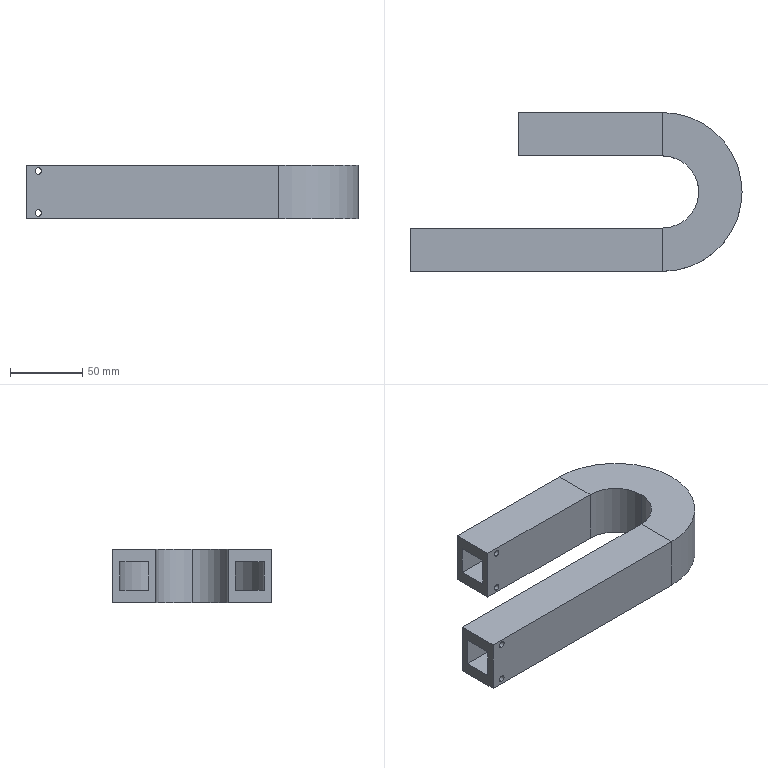Part | SolidWorks | features HoleWzd 2, Sweep 1 | 1 solid | 38 faces | box 230 x 110 x 37 mm | volume 282563 mm3 | plane 22 | cylinder 16 | commonest cylinder face diameters 4.5 x8 50 x2 60 x2 100 x2 110 x2
STEP:
#1=CARTESIAN_POINT('',(83.5,65.,-12.25));
#2=VERTEX_POINT('',#1);
#3=CARTESIAN_POINT('',(83.5,65.,-16.75));
#4=VERTEX_POINT('',#3);
#5=CARTESIAN_POINT('',(83.5,65.,-14.5));
#6=DIRECTION('',(0.,-1.,0.));
#7=DIRECTION('',(1.,0.,0.));
#8=AXIS2_PLACEMENT_3D('',#5,#6,#7);
#9=CIRCLE('',#8,2.25);
#10=EDGE_CURVE('',#2,#4,#9,.T.);
#11=ORIENTED_EDGE('',*,*,#10,.T.);
#12=CARTESIAN_POINT('',(83.5,95.,-16.75));
#13=VERTEX_POINT('',#12);
#14=CARTESIAN_POINT('',(83.5,95.,-16.75));
#15=DIRECTION('',(0.,1.,0.));
#16=VECTOR('',#15,1000.);
#17=LINE('',#14,#16);
#18=EDGE_CURVE('',#4,#13,#17,.T.);
#19=ORIENTED_EDGE('',*,*,#18,.T.);
#20=CARTESIAN_POINT('',(83.5,95.,-12.25));
#21=VERTEX_POINT('',#20);
#22=CARTESIAN_POINT('',(83.5,95.,-14.5));
#23=DIRECTION('',(0.,1.,0.));
#24=DIRECTION('',(0.,0.,1.));
#25=AXIS2_PLACEMENT_3D('',#22,#23,#24);
#26=CIRCLE('',#25,2.25);
#27=EDGE_CURVE('',#13,#21,#26,.T.);
#28=ORIENTED_EDGE('',*,*,#27,.T.);
#29=CARTESIAN_POINT('',(83.5,95.,-12.25));
#30=DIRECTION('',(0.,1.,0.));
#31=VECTOR('',#30,1000.);
#32=LINE('',#29,#31);
#33=EDGE_CURVE('',#2,#21,#32,.T.);
#34=ORIENTED_EDGE('',*,*,#33,.F.);
#35=EDGE_LOOP('',(#11,#19,#28,#34));
#36=FACE_OUTER_BOUND('',#35,.T.);
#37=CARTESIAN_POINT('',(83.5,95.,-14.5));
#38=DIRECTION('',(0.,1.,0.));
#39=DIRECTION('',(0.,0.,1.));
#40=AXIS2_PLACEMENT_3D('',#37,#38,#39);
#41=CYLINDRICAL_SURFACE('',#40,2.25);
#42=ADVANCED_FACE('',(#36),#41,.F.);
#43=CARTESIAN_POINT('',(83.5,65.,16.75));
#44=VERTEX_POINT('',#43);
#45=CARTESIAN_POINT('',(83.5,65.,12.25));
#46=VERTEX_POINT('',#45);
#47=CARTESIAN_POINT('',(83.5,65.,14.5));
#48=DIRECTION('',(0.,-1.,0.));
#49=DIRECTION('',(1.,0.,0.));
#50=AXIS2_PLACEMENT_3D('',#47,#48,#49);
#51=CIRCLE('',#50,2.25);
#52=EDGE_CURVE('',#44,#46,#51,.T.);
#53=ORIENTED_EDGE('',*,*,#52,.T.);
#54=CARTESIAN_POINT('',(83.5,95.,12.25));
#55=VERTEX_POINT('',#54);
#56=CARTESIAN_POINT('',(83.5,95.,12.25));
#57=DIRECTION('',(0.,1.,0.));
#58=VECTOR('',#57,1000.);
#59=LINE('',#56,#58);
#60=EDGE_CURVE('',#46,#55,#59,.T.);
#61=ORIENTED_EDGE('',*,*,#60,.T.);
#62=CARTESIAN_POINT('',(83.5,95.,16.75));
#63=VERTEX_POINT('',#62);
#64=CARTESIAN_POINT('',(83.5,95.,14.5));
#65=DIRECTION('',(0.,1.,0.));
#66=DIRECTION('',(0.,0.,1.));
#67=AXIS2_PLACEMENT_3D('',#64,#65,#66);
#68=CIRCLE('',#67,2.25);
#69=EDGE_CURVE('',#55,#63,#68,.T.);
#70=ORIENTED_EDGE('',*,*,#69,.T.);
#71=CARTESIAN_POINT('',(83.5,95.,16.75));
#72=DIRECTION('',(0.,1.,0.));
#73=VECTOR('',#72,1000.);
#74=LINE('',#71,#73);
#75=EDGE_CURVE('',#44,#63,#74,.T.);
#76=ORIENTED_EDGE('',*,*,#75,.F.);
#77=EDGE_LOOP('',(#53,#61,#70,#76));
#78=FACE_OUTER_BOUND('',#77,.T.);
#79=CARTESIAN_POINT('',(83.5,95.,14.5));
#80=DIRECTION('',(0.,1.,0.));
#81=DIRECTION('',(0.,0.,1.));
#82=AXIS2_PLACEMENT_3D('',#79,#80,#81);
#83=CYLINDRICAL_SURFACE('',#82,2.25);
#84=ADVANCED_FACE('',(#78),#83,.F.);
#85=CARTESIAN_POINT('',(8.5,-15.,-16.75));
#86=VERTEX_POINT('',#85);
#87=CARTESIAN_POINT('',(8.5,-15.,-12.25));
#88=VERTEX_POINT('',#87);
#89=CARTESIAN_POINT('',(8.5,-15.,-14.5));
#90=DIRECTION('',(0.,1.,0.));
#91=DIRECTION('',(0.,0.,1.));
#92=AXIS2_PLACEMENT_3D('',#89,#90,#91);
#93=CIRCLE('',#92,2.25);
#94=EDGE_CURVE('',#86,#88,#93,.T.);
#95=ORIENTED_EDGE('',*,*,#94,.F.);
#96=CARTESIAN_POINT('',(8.5,15.,-16.75));
#97=VERTEX_POINT('',#96);
#98=CARTESIAN_POINT('',(8.5,15.,-16.75));
#99=DIRECTION('',(0.,1.,0.));
#100=VECTOR('',#99,1000.);
#101=LINE('',#98,#100);
#102=EDGE_CURVE('',#86,#97,#101,.T.);
#103=ORIENTED_EDGE('',*,*,#102,.T.);
#104=CARTESIAN_POINT('',(8.5,15.,-12.25));
#105=VERTEX_POINT('',#104);
#106=CARTESIAN_POINT('',(8.5,15.,-14.5));
#107=DIRECTION('',(0.,1.,0.));
#108=DIRECTION('',(0.,0.,1.));
#109=AXIS2_PLACEMENT_3D('',#106,#107,#108);
#110=CIRCLE('',#109,2.25);
#111=EDGE_CURVE('',#97,#105,#110,.T.);
#112=ORIENTED_EDGE('',*,*,#111,.T.);
#113=CARTESIAN_POINT('',(8.5,15.,-12.25));
#114=DIRECTION('',(0.,1.,0.));
#115=VECTOR('',#114,1000.);
#116=LINE('',#113,#115);
#117=EDGE_CURVE('',#88,#105,#116,.T.);
#118=ORIENTED_EDGE('',*,*,#117,.F.);
#119=EDGE_LOOP('',(#95,#103,#112,#118));
#120=FACE_OUTER_BOUND('',#119,.T.);
#121=CARTESIAN_POINT('',(8.5,15.,-14.5));
#122=DIRECTION('',(0.,1.,0.));
#123=DIRECTION('',(0.,0.,1.));
#124=AXIS2_PLACEMENT_3D('',#121,#122,#123);
#125=CYLINDRICAL_SURFACE('',#124,2.25);
#126=ADVANCED_FACE('',(#120),#125,.F.);
#127=CARTESIAN_POINT('',(8.5,-15.,12.25));
#128=VERTEX_POINT('',#127);
#129=CARTESIAN_POINT('',(8.5,-15.,16.75));
#130=VERTEX_POINT('',#129);
#131=CARTESIAN_POINT('',(8.5,-15.,14.5));
#132=DIRECTION('',(0.,1.,0.));
#133=DIRECTION('',(0.,0.,1.));
#134=AXIS2_PLACEMENT_3D('',#131,#132,#133);
#135=CIRCLE('',#134,2.25);
#136=EDGE_CURVE('',#128,#130,#135,.T.);
#137=ORIENTED_EDGE('',*,*,#136,.F.);
#138=CARTESIAN_POINT('',(8.5,15.,12.25));
#139=VERTEX_POINT('',#138);
#140=CARTESIAN_POINT('',(8.5,15.,12.25));
#141=DIRECTION('',(0.,1.,0.));
#142=VECTOR('',#141,1000.);
#143=LINE('',#140,#142);
#144=EDGE_CURVE('',#128,#139,#143,.T.);
#145=ORIENTED_EDGE('',*,*,#144,.T.);
#146=CARTESIAN_POINT('',(8.5,15.,16.75));
#147=VERTEX_POINT('',#146);
#148=CARTESIAN_POINT('',(8.5,15.,14.5));
#149=DIRECTION('',(0.,1.,0.));
#150=DIRECTION('',(0.,0.,1.));
#151=AXIS2_PLACEMENT_3D('',#148,#149,#150);
#152=CIRCLE('',#151,2.25);
#153=EDGE_CURVE('',#139,#147,#152,.T.);
#154=ORIENTED_EDGE('',*,*,#153,.T.);
#155=CARTESIAN_POINT('',(8.5,15.,16.75));
#156=DIRECTION('',(0.,1.,0.));
#157=VECTOR('',#156,1000.);
#158=LINE('',#155,#157);
#159=EDGE_CURVE('',#130,#147,#158,.T.);
#160=ORIENTED_EDGE('',*,*,#159,.F.);
#161=EDGE_LOOP('',(#137,#145,#154,#160));
#162=FACE_OUTER_BOUND('',#161,.T.);
#163=CARTESIAN_POINT('',(8.5,15.,14.5));
#164=DIRECTION('',(0.,1.,0.));
#165=DIRECTION('',(0.,0.,1.));
#166=AXIS2_PLACEMENT_3D('',#163,#164,#165);
#167=CYLINDRICAL_SURFACE('',#166,2.25);
#168=ADVANCED_FACE('',(#162),#167,.F.);
#169=CARTESIAN_POINT('',(175.,10.,-10.));
#170=VERTEX_POINT('',#169);
#171=CARTESIAN_POINT('',(205.,40.,-10.));
#172=VERTEX_POINT('',#171);
#173=CARTESIAN_POINT('',(175.,40.,-10.));
#174=DIRECTION('',(0.,0.,1.));
#175=DIRECTION('',(0.,-1.,0.));
#176=AXIS2_PLACEMENT_3D('',#173,#174,#175);
#177=CIRCLE('',#176,30.);
#178=EDGE_CURVE('',#170,#172,#177,.T.);
#179=ORIENTED_EDGE('',*,*,#178,.T.);
#180=CARTESIAN_POINT('',(205.,40.,10.));
#181=VERTEX_POINT('',#180);
#182=CARTESIAN_POINT('',(205.,40.,0.));
#183=DIRECTION('',(0.,0.,1.));
#184=VECTOR('',#183,1000.);
#185=LINE('',#182,#184);
#186=EDGE_CURVE('',#172,#181,#185,.T.);
#187=ORIENTED_EDGE('',*,*,#186,.T.);
#188=CARTESIAN_POINT('',(175.,10.,10.));
#189=VERTEX_POINT('',#188);
#190=CARTESIAN_POINT('',(175.,40.,10.));
#191=DIRECTION('',(0.,0.,1.));
#192=DIRECTION('',(0.,-1.,0.));
#193=AXIS2_PLACEMENT_3D('',#190,#191,#192);
#194=CIRCLE('',#193,30.);
#195=EDGE_CURVE('',#189,#181,#194,.T.);
#196=ORIENTED_EDGE('',*,*,#195,.F.);
#197=CARTESIAN_POINT('',(175.,10.,10.));
#198=DIRECTION('',(0.,0.,-1.));
#199=VECTOR('',#198,1000.);
#200=LINE('',#197,#199);
#201=EDGE_CURVE('',#189,#170,#200,.T.);
#202=ORIENTED_EDGE('',*,*,#201,.T.);
#203=EDGE_LOOP('',(#179,#187,#196,#202));
#204=FACE_OUTER_BOUND('',#203,.T.);
#205=CARTESIAN_POINT('',(175.,40.,0.));
#206=DIRECTION('',(0.,0.,1.));
#207=DIRECTION('',(1.,0.,0.));
#208=AXIS2_PLACEMENT_3D('',#205,#206,#207);
#209=CYLINDRICAL_SURFACE('',#208,30.);
#210=ADVANCED_FACE('',(#204),#209,.T.);
#211=CARTESIAN_POINT('',(225.,40.,-10.));
#212=VERTEX_POINT('',#211);
#213=CARTESIAN_POINT('',(175.,90.,-10.));
#214=VERTEX_POINT('',#213);
#215=CARTESIAN_POINT('',(175.,40.,-10.));
#216=DIRECTION('',(0.,0.,1.));
#217=DIRECTION('',(0.,-1.,0.));
#218=AXIS2_PLACEMENT_3D('',#215,#216,#217);
#219=CIRCLE('',#218,50.);
#220=EDGE_CURVE('',#212,#214,#219,.T.);
#221=ORIENTED_EDGE('',*,*,#220,.F.);
#222=CARTESIAN_POINT('',(225.,40.,10.));
#223=VERTEX_POINT('',#222);
#224=CARTESIAN_POINT('',(225.,40.,0.));
#225=DIRECTION('',(0.,0.,1.));
#226=VECTOR('',#225,1000.);
#227=LINE('',#224,#226);
#228=EDGE_CURVE('',#212,#223,#227,.T.);
#229=ORIENTED_EDGE('',*,*,#228,.T.);
#230=CARTESIAN_POINT('',(175.,90.,10.));
#231=VERTEX_POINT('',#230);
#232=CARTESIAN_POINT('',(175.,40.,10.));
#233=DIRECTION('',(0.,0.,1.));
#234=DIRECTION('',(0.,-1.,0.));
#235=AXIS2_PLACEMENT_3D('',#232,#233,#234);
#236=CIRCLE('',#235,50.);
#237=EDGE_CURVE('',#223,#231,#236,.T.);
#238=ORIENTED_EDGE('',*,*,#237,.T.);
#239=CARTESIAN_POINT('',(175.,90.,10.));
#240=DIRECTION('',(0.,0.,1.));
#241=VECTOR('',#240,1000.);
#242=LINE('',#239,#241);
#243=EDGE_CURVE('',#214,#231,#242,.T.);
#244=ORIENTED_EDGE('',*,*,#243,.F.);
#245=EDGE_LOOP('',(#221,#229,#238,#244));
#246=FACE_OUTER_BOUND('',#245,.T.);
#247=CARTESIAN_POINT('',(175.,40.,0.));
#248=DIRECTION('',(0.,0.,1.));
#249=DIRECTION('',(1.,0.,0.));
#250=AXIS2_PLACEMENT_3D('',#247,#248,#249);
#251=CYLINDRICAL_SURFACE('',#250,50.);
#252=ADVANCED_FACE('',(#246),#251,.F.);
#253=CARTESIAN_POINT('',(175.,-15.,-18.5));
#254=VERTEX_POINT('',#253);
#255=CARTESIAN_POINT('',(230.,40.,-18.5));
#256=VERTEX_POINT('',#255);
#257=CARTESIAN_POINT('',(175.,40.,-18.5));
#258=DIRECTION('',(0.,0.,1.));
#259=DIRECTION('',(0.,-1.,0.));
#260=AXIS2_PLACEMENT_3D('',#257,#258,#259);
#261=CIRCLE('',#260,55.);
#262=EDGE_CURVE('',#254,#256,#261,.T.);
#263=ORIENTED_EDGE('',*,*,#262,.T.);
#264=CARTESIAN_POINT('',(230.,40.,18.5));
#265=VERTEX_POINT('',#264);
#266=CARTESIAN_POINT('',(230.,40.,0.));
#267=DIRECTION('',(0.,0.,1.));
#268=VECTOR('',#267,1000.);
#269=LINE('',#266,#268);
#270=EDGE_CURVE('',#256,#265,#269,.T.);
#271=ORIENTED_EDGE('',*,*,#270,.T.);
#272=CARTESIAN_POINT('',(175.,-15.,18.5));
#273=VERTEX_POINT('',#272);
#274=CARTESIAN_POINT('',(175.,40.,18.5));
#275=DIRECTION('',(0.,0.,1.));
#276=DIRECTION('',(0.,-1.,0.));
#277=AXIS2_PLACEMENT_3D('',#274,#275,#276);
#278=CIRCLE('',#277,55.);
#279=EDGE_CURVE('',#273,#265,#278,.T.);
#280=ORIENTED_EDGE('',*,*,#279,.F.);
#281=CARTESIAN_POINT('',(175.,-15.,18.5));
#282=DIRECTION('',(0.,0.,-1.));
#283=VECTOR('',#282,1000.);
#284=LINE('',#281,#283);
#285=EDGE_CURVE('',#273,#254,#284,.T.);
#286=ORIENTED_EDGE('',*,*,#285,.T.);
#287=EDGE_LOOP('',(#263,#271,#280,#286));
#288=FACE_OUTER_BOUND('',#287,.T.);
#289=CARTESIAN_POINT('',(175.,40.,0.));
#290=DIRECTION('',(0.,0.,1.));
#291=DIRECTION('',(1.,0.,0.));
#292=AXIS2_PLACEMENT_3D('',#289,#290,#291);
#293=CYLINDRICAL_SURFACE('',#292,55.);
#294=ADVANCED_FACE('',(#288),#293,.T.);
#295=CARTESIAN_POINT('',(200.,40.,-18.5));
#296=VERTEX_POINT('',#295);
#297=CARTESIAN_POINT('',(175.,65.,-18.5));
#298=VERTEX_POINT('',#297);
#299=CARTESIAN_POINT('',(175.,40.,-18.5));
#300=DIRECTION('',(0.,0.,1.));
#301=DIRECTION('',(0.,-1.,0.));
#302=AXIS2_PLACEMENT_3D('',#299,#300,#301);
#303=CIRCLE('',#302,25.);
#304=EDGE_CURVE('',#296,#298,#303,.T.);
#305=ORIENTED_EDGE('',*,*,#304,.F.);
#306=CARTESIAN_POINT('',(200.,40.,18.5));
#307=VERTEX_POINT('',#306);
#308=CARTESIAN_POINT('',(200.,40.,0.));
#309=DIRECTION('',(0.,0.,1.));
#310=VECTOR('',#309,1000.);
#311=LINE('',#308,#310);
#312=EDGE_CURVE('',#296,#307,#311,.T.);
#313=ORIENTED_EDGE('',*,*,#312,.T.);
#314=CARTESIAN_POINT('',(175.,65.,18.5));
#315=VERTEX_POINT('',#314);
#316=CARTESIAN_POINT('',(175.,40.,18.5));
#317=DIRECTION('',(0.,0.,1.));
#318=DIRECTION('',(0.,-1.,0.));
#319=AXIS2_PLACEMENT_3D('',#316,#317,#318);
#320=CIRCLE('',#319,25.);
#321=EDGE_CURVE('',#307,#315,#320,.T.);
#322=ORIENTED_EDGE('',*,*,#321,.T.);
#323=CARTESIAN_POINT('',(175.,65.,18.5));
#324=DIRECTION('',(0.,0.,1.));
#325=VECTOR('',#324,1000.);
#326=LINE('',#323,#325);
#327=EDGE_CURVE('',#298,#315,#326,.T.);
#328=ORIENTED_EDGE('',*,*,#327,.F.);
#329=EDGE_LOOP('',(#305,#313,#322,#328));
#330=FACE_OUTER_BOUND('',#329,.T.);
#331=CARTESIAN_POINT('',(175.,40.,0.));
#332=DIRECTION('',(0.,0.,1.));
#333=DIRECTION('',(1.,0.,0.));
#334=AXIS2_PLACEMENT_3D('',#331,#332,#333);
#335=CYLINDRICAL_SURFACE('',#334,25.);
#336=ADVANCED_FACE('',(#330),#335,.F.);
#337=CARTESIAN_POINT('',(75.,70.,-10.));
#338=VERTEX_POINT('',#337);
#339=CARTESIAN_POINT('',(75.,90.,-10.));
#340=VERTEX_POINT('',#339);
#341=CARTESIAN_POINT('',(75.,90.,-10.));
#342=DIRECTION('',(0.,1.,0.));
#343=VECTOR('',#342,1000.);
#344=LINE('',#341,#343);
#345=EDGE_CURVE('',#338,#340,#344,.T.);
#346=ORIENTED_EDGE('',*,*,#345,.F.);
#347=CARTESIAN_POINT('',(175.,70.,-10.));
#348=VERTEX_POINT('',#347);
#349=CARTESIAN_POINT('',(175.,70.,-10.));
#350=DIRECTION('',(-1.,0.,0.));
#351=VECTOR('',#350,1000.);
#352=LINE('',#349,#351);
#353=EDGE_CURVE('',#348,#338,#352,.T.);
#354=ORIENTED_EDGE('',*,*,#353,.F.);
#355=CARTESIAN_POINT('',(175.,90.,-10.));
#356=DIRECTION('',(0.,1.,0.));
#357=VECTOR('',#356,1000.);
#358=LINE('',#355,#357);
#359=EDGE_CURVE('',#348,#214,#358,.T.);
#360=ORIENTED_EDGE('',*,*,#359,.T.);
#361=CARTESIAN_POINT('',(175.,90.,-10.));
#362=DIRECTION('',(-1.,0.,0.));
#363=VECTOR('',#362,1000.);
#364=LINE('',#361,#363);
#365=EDGE_CURVE('',#214,#340,#364,.T.);
#366=ORIENTED_EDGE('',*,*,#365,.T.);
#367=EDGE_LOOP('',(#346,#354,#360,#366));
#368=FACE_OUTER_BOUND('',#367,.T.);
#369=CARTESIAN_POINT('',(175.,90.,-10.));
#370=DIRECTION('',(0.,0.,1.));
#371=DIRECTION('',(1.,0.,0.));
#372=AXIS2_PLACEMENT_3D('',#369,#370,#371);
#373=PLANE('',#372);
#374=ADVANCED_FACE('',(#368),#373,.T.);
#375=ORIENTED_EDGE('',*,*,#353,.T.);
#376=CARTESIAN_POINT('',(75.,70.,10.));
#377=VERTEX_POINT('',#376);
#378=CARTESIAN_POINT('',(75.,70.,10.));
#379=DIRECTION('',(0.,0.,-1.));
#380=VECTOR('',#379,1000.);
#381=LINE('',#378,#380);
#382=EDGE_CURVE('',#377,#338,#381,.T.);
#383=ORIENTED_EDGE('',*,*,#382,.F.);
#384=CARTESIAN_POINT('',(175.,70.,10.));
#385=VERTEX_POINT('',#384);
#386=CARTESIAN_POINT('',(175.,70.,10.));
#387=DIRECTION('',(-1.,0.,0.));
#388=VECTOR('',#387,1000.);
#389=LINE('',#386,#388);
#390=EDGE_CURVE('',#385,#377,#389,.T.);
#391=ORIENTED_EDGE('',*,*,#390,.F.);
#392=CARTESIAN_POINT('',(175.,70.,10.));
#393=DIRECTION('',(0.,0.,-1.));
#394=VECTOR('',#393,1000.);
#395=LINE('',#392,#394);
#396=EDGE_CURVE('',#385,#348,#395,.T.);
#397=ORIENTED_EDGE('',*,*,#396,.T.);
#398=EDGE_LOOP('',(#375,#383,#391,#397));
#399=FACE_OUTER_BOUND('',#398,.T.);
#400=CARTESIAN_POINT('',(175.,70.,10.));
#401=DIRECTION('',(0.,1.,0.));
#402=DIRECTION('',(-1.,0.,0.));
#403=AXIS2_PLACEMENT_3D('',#400,#401,#402);
#404=PLANE('',#403);
#405=ADVANCED_FACE('',(#399),#404,.T.);
#406=ORIENTED_EDGE('',*,*,#390,.T.);
#407=CARTESIAN_POINT('',(75.,90.,10.));
#408=VERTEX_POINT('',#407);
#409=CARTESIAN_POINT('',(75.,90.,10.));
#410=DIRECTION('',(0.,-1.,0.));
#411=VECTOR('',#410,1000.);
#412=LINE('',#409,#411);
#413=EDGE_CURVE('',#408,#377,#412,.T.);
#414=ORIENTED_EDGE('',*,*,#413,.F.);
#415=CARTESIAN_POINT('',(175.,90.,10.));
#416=DIRECTION('',(-1.,0.,0.));
#417=VECTOR('',#416,1000.);
#418=LINE('',#415,#417);
#419=EDGE_CURVE('',#231,#408,#418,.T.);
#420=ORIENTED_EDGE('',*,*,#419,.F.);
#421=CARTESIAN_POINT('',(175.,90.,10.));
#422=DIRECTION('',(0.,-1.,0.));
#423=VECTOR('',#422,1000.);
#424=LINE('',#421,#423);
#425=EDGE_CURVE('',#231,#385,#424,.T.);
#426=ORIENTED_EDGE('',*,*,#425,.T.);
#427=EDGE_LOOP('',(#406,#414,#420,#426));
#428=FACE_OUTER_BOUND('',#427,.T.);
#429=CARTESIAN_POINT('',(175.,90.,10.));
#430=DIRECTION('',(0.,0.,-1.));
#431=DIRECTION('',(-1.,0.,0.));
#432=AXIS2_PLACEMENT_3D('',#429,#430,#431);
#433=PLANE('',#432);
#434=ADVANCED_FACE('',(#428),#433,.T.);
#435=ORIENTED_EDGE('',*,*,#419,.T.);
#436=CARTESIAN_POINT('',(75.,90.,10.));
#437=DIRECTION('',(0.,0.,1.));
#438=VECTOR('',#437,1000.);
#439=LINE('',#436,#438);
#440=EDGE_CURVE('',#340,#408,#439,.T.);
#441=ORIENTED_EDGE('',*,*,#440,.F.);
#442=ORIENTED_EDGE('',*,*,#365,.F.);
#443=ORIENTED_EDGE('',*,*,#243,.T.);
#444=EDGE_LOOP('',(#435,#441,#442,#443));
#445=FACE_OUTER_BOUND('',#444,.T.);
#446=CARTESIAN_POINT('',(175.,90.,10.));
#447=DIRECTION('',(0.,-1.,0.));
#448=DIRECTION('',(1.,0.,0.));
#449=AXIS2_PLACEMENT_3D('',#446,#447,#448);
#450=PLANE('',#449);
#451=ADVANCED_FACE('',(#445),#450,.T.);
#452=ORIENTED_EDGE('',*,*,#359,.F.);
#453=CARTESIAN_POINT('',(175.,40.,-10.));
#454=DIRECTION('',(0.,0.,1.));
#455=DIRECTION('',(0.,-1.,0.));
#456=AXIS2_PLACEMENT_3D('',#453,#454,#455);
#457=CIRCLE('',#456,30.);
#458=EDGE_CURVE('',#172,#348,#457,.T.);
#459=ORIENTED_EDGE('',*,*,#458,.F.);
#460=ORIENTED_EDGE('',*,*,#178,.F.);
#461=CARTESIAN_POINT('',(175.,-10.,-10.));
#462=VERTEX_POINT('',#461);
#463=CARTESIAN_POINT('',(175.,-10.,-10.));
#464=DIRECTION('',(0.,-1.,0.));
#465=VECTOR('',#464,1000.);
#466=LINE('',#463,#465);
#467=EDGE_CURVE('',#170,#462,#466,.T.);
#468=ORIENTED_EDGE('',*,*,#467,.T.);
#469=CARTESIAN_POINT('',(175.,40.,-10.));
#470=DIRECTION('',(0.,0.,1.));
#471=DIRECTION('',(0.,-1.,0.));
#472=AXIS2_PLACEMENT_3D('',#469,#470,#471);
#473=CIRCLE('',#472,50.);
#474=EDGE_CURVE('',#462,#212,#473,.T.);
#475=ORIENTED_EDGE('',*,*,#474,.T.);
#476=ORIENTED_EDGE('',*,*,#220,.T.);
#477=EDGE_LOOP('',(#452,#459,#460,#468,#475,#476));
#478=FACE_OUTER_BOUND('',#477,.T.);
#479=CARTESIAN_POINT('',(175.,-10.,-10.));
#480=DIRECTION('',(0.,0.,1.));
#481=DIRECTION('',(1.,0.,0.));
#482=AXIS2_PLACEMENT_3D('',#479,#480,#481);
#483=PLANE('',#482);
#484=ADVANCED_FACE('',(#478),#483,.T.);
#485=ORIENTED_EDGE('',*,*,#186,.F.);
#486=ORIENTED_EDGE('',*,*,#458,.T.);
#487=ORIENTED_EDGE('',*,*,#396,.F.);
#488=CARTESIAN_POINT('',(175.,40.,10.));
#489=DIRECTION('',(0.,0.,1.));
#490=DIRECTION('',(0.,-1.,0.));
#491=AXIS2_PLACEMENT_3D('',#488,#489,#490);
#492=CIRCLE('',#491,30.);
#493=EDGE_CURVE('',#181,#385,#492,.T.);
#494=ORIENTED_EDGE('',*,*,#493,.F.);
#495=EDGE_LOOP('',(#485,#486,#487,#494));
#496=FACE_OUTER_BOUND('',#495,.T.);
#497=CARTESIAN_POINT('',(175.,40.,0.));
#498=DIRECTION('',(0.,0.,1.));
#499=DIRECTION('',(1.,0.,0.));
#500=AXIS2_PLACEMENT_3D('',#497,#498,#499);
#501=CYLINDRICAL_SURFACE('',#500,30.);
#502=ADVANCED_FACE('',(#496),#501,.T.);
#503=ORIENTED_EDGE('',*,*,#195,.T.);
#504=ORIENTED_EDGE('',*,*,#493,.T.);
#505=ORIENTED_EDGE('',*,*,#425,.F.);
#506=ORIENTED_EDGE('',*,*,#237,.F.);
#507=CARTESIAN_POINT('',(175.,-10.,10.));
#508=VERTEX_POINT('',#507);
#509=CARTESIAN_POINT('',(175.,40.,10.));
#510=DIRECTION('',(0.,0.,1.));
#511=DIRECTION('',(0.,-1.,0.));
#512=AXIS2_PLACEMENT_3D('',#509,#510,#511);
#513=CIRCLE('',#512,50.);
#514=EDGE_CURVE('',#508,#223,#513,.T.);
#515=ORIENTED_EDGE('',*,*,#514,.F.);
#516=CARTESIAN_POINT('',(175.,-10.,10.));
#517=DIRECTION('',(0.,1.,0.));
#518=VECTOR('',#517,1000.);
#519=LINE('',#516,#518);
#520=EDGE_CURVE('',#508,#189,#519,.T.);
#521=ORIENTED_EDGE('',*,*,#520,.T.);
#522=EDGE_LOOP('',(#503,#504,#505,#506,#515,#521));
#523=FACE_OUTER_BOUND('',#522,.T.);
#524=CARTESIAN_POINT('',(175.,-10.,10.));
#525=DIRECTION('',(0.,0.,-1.));
#526=DIRECTION('',(-1.,0.,0.));
#527=AXIS2_PLACEMENT_3D('',#524,#525,#526);
#528=PLANE('',#527);
#529=ADVANCED_FACE('',(#523),#528,.T.);
#530=ORIENTED_EDGE('',*,*,#228,.F.);
#531=ORIENTED_EDGE('',*,*,#474,.F.);
#532=CARTESIAN_POINT('',(175.,-10.,10.));
#533=DIRECTION('',(0.,0.,1.));
#534=VECTOR('',#533,1000.);
#535=LINE('',#532,#534);
#536=EDGE_CURVE('',#462,#508,#535,.T.);
#537=ORIENTED_EDGE('',*,*,#536,.T.);
#538=ORIENTED_EDGE('',*,*,#514,.T.);
#539=EDGE_LOOP('',(#530,#531,#537,#538));
#540=FACE_OUTER_BOUND('',#539,.T.);
#541=CARTESIAN_POINT('',(175.,40.,0.));
#542=DIRECTION('',(0.,0.,1.));
#543=DIRECTION('',(1.,0.,0.));
#544=AXIS2_PLACEMENT_3D('',#541,#542,#543);
#545=CYLINDRICAL_SURFACE('',#544,50.);
#546=ADVANCED_FACE('',(#540),#545,.F.);
#547=ORIENTED_EDGE('',*,*,#467,.F.);
#548=CARTESIAN_POINT('',(0.,10.,-10.));
#549=VERTEX_POINT('',#548);
#550=CARTESIAN_POINT('',(0.,10.,-10.));
#551=DIRECTION('',(1.,0.,0.));
#552=VECTOR('',#551,1000.);
#553=LINE('',#550,#552);
#554=EDGE_CURVE('',#549,#170,#553,.T.);
#555=ORIENTED_EDGE('',*,*,#554,.F.);
#556=CARTESIAN_POINT('',(0.,-10.,-10.));
#557=VERTEX_POINT('',#556);
#558=CARTESIAN_POINT('',(0.,-10.,-10.));
#559=DIRECTION('',(0.,-1.,0.));
#560=VECTOR('',#559,1000.);
#561=LINE('',#558,#560);
#562=EDGE_CURVE('',#549,#557,#561,.T.);
#563=ORIENTED_EDGE('',*,*,#562,.T.);
#564=CARTESIAN_POINT('',(0.,-10.,-10.));
#565=DIRECTION('',(1.,0.,0.));
#566=VECTOR('',#565,1000.);
#567=LINE('',#564,#566);
#568=EDGE_CURVE('',#557,#462,#567,.T.);
#569=ORIENTED_EDGE('',*,*,#568,.T.);
#570=EDGE_LOOP('',(#547,#555,#563,#569));
#571=FACE_OUTER_BOUND('',#570,.T.);
#572=CARTESIAN_POINT('',(0.,-10.,-10.));
#573=DIRECTION('',(0.,0.,1.));
#574=DIRECTION('',(1.,0.,0.));
#575=AXIS2_PLACEMENT_3D('',#572,#573,#574);
#576=PLANE('',#575);
#577=ADVANCED_FACE('',(#571),#576,.T.);
#578=ORIENTED_EDGE('',*,*,#554,.T.);
#579=ORIENTED_EDGE('',*,*,#201,.F.);
#580=CARTESIAN_POINT('',(0.,10.,10.));
#581=VERTEX_POINT('',#580);
#582=CARTESIAN_POINT('',(0.,10.,10.));
#583=DIRECTION('',(1.,0.,0.));
#584=VECTOR('',#583,1000.);
#585=LINE('',#582,#584);
#586=EDGE_CURVE('',#581,#189,#585,.T.);
#587=ORIENTED_EDGE('',*,*,#586,.F.);
#588=CARTESIAN_POINT('',(0.,10.,10.));
#589=DIRECTION('',(0.,0.,-1.));
#590=VECTOR('',#589,1000.);
#591=LINE('',#588,#590);
#592=EDGE_CURVE('',#581,#549,#591,.T.);
#593=ORIENTED_EDGE('',*,*,#592,.T.);
#594=EDGE_LOOP('',(#578,#579,#587,#593));
#595=FACE_OUTER_BOUND('',#594,.T.);
#596=CARTESIAN_POINT('',(0.,10.,10.));
#597=DIRECTION('',(0.,-1.,0.));
#598=DIRECTION('',(0.,0.,-1.));
#599=AXIS2_PLACEMENT_3D('',#596,#597,#598);
#600=PLANE('',#599);
#601=ADVANCED_FACE('',(#595),#600,.T.);
#602=ORIENTED_EDGE('',*,*,#586,.T.);
#603=ORIENTED_EDGE('',*,*,#520,.F.);
#604=CARTESIAN_POINT('',(0.,-10.,10.));
#605=VERTEX_POINT('',#604);
#606=CARTESIAN_POINT('',(0.,-10.,10.));
#607=DIRECTION('',(1.,0.,0.));
#608=VECTOR('',#607,1000.);
#609=LINE('',#606,#608);
#610=EDGE_CURVE('',#605,#508,#609,.T.);
#611=ORIENTED_EDGE('',*,*,#610,.F.);
#612=CARTESIAN_POINT('',(0.,-10.,10.));
#613=DIRECTION('',(0.,1.,0.));
#614=VECTOR('',#613,1000.);
#615=LINE('',#612,#614);
#616=EDGE_CURVE('',#605,#581,#615,.T.);
#617=ORIENTED_EDGE('',*,*,#616,.T.);
#618=EDGE_LOOP('',(#602,#603,#611,#617));
#619=FACE_OUTER_BOUND('',#618,.T.);
#620=CARTESIAN_POINT('',(0.,-10.,10.));
#621=DIRECTION('',(0.,0.,-1.));
#622=DIRECTION('',(-1.,0.,0.));
#623=AXIS2_PLACEMENT_3D('',#620,#621,#622);
#624=PLANE('',#623);
#625=ADVANCED_FACE('',(#619),#624,.T.);
#626=ORIENTED_EDGE('',*,*,#610,.T.);
#627=ORIENTED_EDGE('',*,*,#536,.F.);
#628=ORIENTED_EDGE('',*,*,#568,.F.);
#629=CARTESIAN_POINT('',(0.,-10.,10.));
#630=DIRECTION('',(0.,0.,1.));
#631=VECTOR('',#630,1000.);
#632=LINE('',#629,#631);
#633=EDGE_CURVE('',#557,#605,#632,.T.);
#634=ORIENTED_EDGE('',*,*,#633,.T.);
#635=EDGE_LOOP('',(#626,#627,#628,#634));
#636=FACE_OUTER_BOUND('',#635,.T.);
#637=CARTESIAN_POINT('',(0.,-10.,10.));
#638=DIRECTION('',(0.,1.,0.));
#639=DIRECTION('',(0.,0.,1.));
#640=AXIS2_PLACEMENT_3D('',#637,#638,#639);
#641=PLANE('',#640);
#642=ADVANCED_FACE('',(#636),#641,.T.);
#643=CARTESIAN_POINT('',(75.,95.,-18.5));
#644=VERTEX_POINT('',#643);
#645=CARTESIAN_POINT('',(75.,65.,-18.5));
#646=VERTEX_POINT('',#645);
#647=CARTESIAN_POINT('',(75.,95.,-18.5));
#648=DIRECTION('',(0.,-1.,0.));
#649=VECTOR('',#648,1000.);
#650=LINE('',#647,#649);
#651=EDGE_CURVE('',#644,#646,#650,.T.);
#652=ORIENTED_EDGE('',*,*,#651,.T.);
#653=CARTESIAN_POINT('',(75.,65.,18.5));
#654=VERTEX_POINT('',#653);
#655=CARTESIAN_POINT('',(75.,65.,18.5));
#656=DIRECTION('',(0.,0.,1.));
#657=VECTOR('',#656,1000.);
#658=LINE('',#655,#657);
#659=EDGE_CURVE('',#646,#654,#658,.T.);
#660=ORIENTED_EDGE('',*,*,#659,.T.);
#661=CARTESIAN_POINT('',(75.,95.,18.5));
#662=VERTEX_POINT('',#661);
#663=CARTESIAN_POINT('',(75.,95.,18.5));
#664=DIRECTION('',(0.,1.,0.));
#665=VECTOR('',#664,1000.);
#666=LINE('',#663,#665);
#667=EDGE_CURVE('',#654,#662,#666,.T.);
#668=ORIENTED_EDGE('',*,*,#667,.T.);
#669=CARTESIAN_POINT('',(75.,95.,18.5));
#670=DIRECTION('',(0.,0.,-1.));
#671=VECTOR('',#670,1000.);
#672=LINE('',#669,#671);
#673=EDGE_CURVE('',#662,#644,#672,.T.);
#674=ORIENTED_EDGE('',*,*,#673,.T.);
#675=EDGE_LOOP('',(#652,#660,#668,#674));
#676=FACE_OUTER_BOUND('',#675,.T.);
#677=ORIENTED_EDGE('',*,*,#345,.T.);
#678=ORIENTED_EDGE('',*,*,#440,.T.);
#679=ORIENTED_EDGE('',*,*,#413,.T.);
#680=ORIENTED_EDGE('',*,*,#382,.T.);
#681=EDGE_LOOP('',(#677,#678,#679,#680));
#682=FACE_BOUND('',#681,.T.);
#683=CARTESIAN_POINT('',(75.,80.,0.));
#684=DIRECTION('',(1.,0.,0.));
#685=DIRECTION('',(0.,0.,1.));
#686=AXIS2_PLACEMENT_3D('',#683,#684,#685);
#687=PLANE('',#686);
#688=ADVANCED_FACE('',(#676,#682),#687,.F.);
#689=CARTESIAN_POINT('',(0.,-15.,-18.5));
#690=VERTEX_POINT('',#689);
#691=CARTESIAN_POINT('',(0.,15.,-18.5));
#692=VERTEX_POINT('',#691);
#693=CARTESIAN_POINT('',(0.,-15.,-18.5));
#694=DIRECTION('',(0.,1.,0.));
#695=VECTOR('',#694,1000.);
#696=LINE('',#693,#695);
#697=EDGE_CURVE('',#690,#692,#696,.T.);
#698=ORIENTED_EDGE('',*,*,#697,.F.);
#699=CARTESIAN_POINT('',(0.,-15.,18.5));
#700=VERTEX_POINT('',#699);
#701=CARTESIAN_POINT('',(0.,-15.,18.5));
#702=DIRECTION('',(0.,0.,-1.));
#703=VECTOR('',#702,1000.);
#704=LINE('',#701,#703);
#705=EDGE_CURVE('',#700,#690,#704,.T.);
#706=ORIENTED_EDGE('',*,*,#705,.F.);
#707=CARTESIAN_POINT('',(0.,15.,18.5));
#708=VERTEX_POINT('',#707);
#709=CARTESIAN_POINT('',(0.,-15.,18.5));
#710=DIRECTION('',(0.,-1.,0.));
#711=VECTOR('',#710,1000.);
#712=LINE('',#709,#711);
#713=EDGE_CURVE('',#708,#700,#712,.T.);
#714=ORIENTED_EDGE('',*,*,#713,.F.);
#715=CARTESIAN_POINT('',(0.,15.,18.5));
#716=DIRECTION('',(0.,0.,1.));
#717=VECTOR('',#716,1000.);
#718=LINE('',#715,#717);
#719=EDGE_CURVE('',#692,#708,#718,.T.);
#720=ORIENTED_EDGE('',*,*,#719,.F.);
#721=EDGE_LOOP('',(#698,#706,#714,#720));
#722=FACE_OUTER_BOUND('',#721,.T.);
#723=ORIENTED_EDGE('',*,*,#562,.F.);
#724=ORIENTED_EDGE('',*,*,#592,.F.);
#725=ORIENTED_EDGE('',*,*,#616,.F.);
#726=ORIENTED_EDGE('',*,*,#633,.F.);
#727=EDGE_LOOP('',(#723,#724,#725,#726));
#728=FACE_BOUND('',#727,.T.);
#729=CARTESIAN_POINT('',(0.,0.,0.));
#730=DIRECTION('',(-1.,0.,0.));
#731=DIRECTION('',(0.,0.,1.));
#732=AXIS2_PLACEMENT_3D('',#729,#730,#731);
#733=PLANE('',#732);
#734=ADVANCED_FACE('',(#722,#728),#733,.T.);
#735=CARTESIAN_POINT('',(83.5,95.,-14.5));
#736=DIRECTION('',(0.,1.,0.));
#737=DIRECTION('',(0.,0.,1.));
#738=AXIS2_PLACEMENT_3D('',#735,#736,#737);
#739=CIRCLE('',#738,2.25);
#740=EDGE_CURVE('',#21,#13,#739,.T.);
#741=ORIENTED_EDGE('',*,*,#740,.F.);
#742=ORIENTED_EDGE('',*,*,#27,.F.);
#743=EDGE_LOOP('',(#741,#742));
#744=FACE_BOUND('',#743,.T.);
#745=CARTESIAN_POINT('',(83.5,95.,14.5));
#746=DIRECTION('',(0.,1.,0.));
#747=DIRECTION('',(0.,0.,1.));
#748=AXIS2_PLACEMENT_3D('',#745,#746,#747);
#749=CIRCLE('',#748,2.25);
#750=EDGE_CURVE('',#63,#55,#749,.T.);
#751=ORIENTED_EDGE('',*,*,#750,.F.);
#752=ORIENTED_EDGE('',*,*,#69,.F.);
#753=EDGE_LOOP('',(#751,#752));
#754=FACE_BOUND('',#753,.T.);
#755=ORIENTED_EDGE('',*,*,#673,.F.);
#756=CARTESIAN_POINT('',(175.,95.,18.5));
#757=VERTEX_POINT('',#756);
#758=CARTESIAN_POINT('',(175.,95.,18.5));
#759=DIRECTION('',(-1.,0.,0.));
#760=VECTOR('',#759,1000.);
#761=LINE('',#758,#760);
#762=EDGE_CURVE('',#757,#662,#761,.T.);
#763=ORIENTED_EDGE('',*,*,#762,.F.);
#764=CARTESIAN_POINT('',(175.,95.,-18.5));
#765=VERTEX_POINT('',#764);
#766=CARTESIAN_POINT('',(175.,95.,18.5));
#767=DIRECTION('',(0.,0.,-1.));
#768=VECTOR('',#767,1000.);
#769=LINE('',#766,#768);
#770=EDGE_CURVE('',#757,#765,#769,.T.);
#771=ORIENTED_EDGE('',*,*,#770,.T.);
#772=CARTESIAN_POINT('',(175.,95.,-18.5));
#773=DIRECTION('',(-1.,0.,0.));
#774=VECTOR('',#773,1000.);
#775=LINE('',#772,#774);
#776=EDGE_CURVE('',#765,#644,#775,.T.);
#777=ORIENTED_EDGE('',*,*,#776,.T.);
#778=EDGE_LOOP('',(#755,#763,#771,#777));
#779=FACE_OUTER_BOUND('',#778,.T.);
#780=CARTESIAN_POINT('',(175.,95.,18.5));
#781=DIRECTION('',(0.,1.,0.));
#782=DIRECTION('',(-1.,0.,0.));
#783=AXIS2_PLACEMENT_3D('',#780,#781,#782);
#784=PLANE('',#783);
#785=ADVANCED_FACE('',(#744,#754,#779),#784,.T.);
#786=ORIENTED_EDGE('',*,*,#762,.T.);
#787=ORIENTED_EDGE('',*,*,#667,.F.);
#788=CARTESIAN_POINT('',(175.,65.,18.5));
#789=DIRECTION('',(-1.,0.,0.));
#790=VECTOR('',#789,1000.);
#791=LINE('',#788,#790);
#792=EDGE_CURVE('',#315,#654,#791,.T.);
#793=ORIENTED_EDGE('',*,*,#792,.F.);
#794=CARTESIAN_POINT('',(175.,95.,18.5));
#795=DIRECTION('',(0.,1.,0.));
#796=VECTOR('',#795,1000.);
#797=LINE('',#794,#796);
#798=EDGE_CURVE('',#315,#757,#797,.T.);
#799=ORIENTED_EDGE('',*,*,#798,.T.);
#800=EDGE_LOOP('',(#786,#787,#793,#799));
#801=FACE_OUTER_BOUND('',#800,.T.);
#802=CARTESIAN_POINT('',(175.,95.,18.5));
#803=DIRECTION('',(0.,0.,1.));
#804=DIRECTION('',(1.,0.,0.));
#805=AXIS2_PLACEMENT_3D('',#802,#803,#804);
#806=PLANE('',#805);
#807=ADVANCED_FACE('',(#801),#806,.T.);
#808=ORIENTED_EDGE('',*,*,#10,.F.);
#809=CARTESIAN_POINT('',(83.5,65.,-14.5));
#810=DIRECTION('',(0.,-1.,0.));
#811=DIRECTION('',(1.,0.,0.));
#812=AXIS2_PLACEMENT_3D('',#809,#810,#811);
#813=CIRCLE('',#812,2.25);
#814=EDGE_CURVE('',#4,#2,#813,.T.);
#815=ORIENTED_EDGE('',*,*,#814,.F.);
#816=EDGE_LOOP('',(#808,#815));
#817=FACE_BOUND('',#816,.T.);
#818=ORIENTED_EDGE('',*,*,#52,.F.);
#819=CARTESIAN_POINT('',(83.5,65.,14.5));
#820=DIRECTION('',(0.,-1.,0.));
#821=DIRECTION('',(1.,0.,0.));
#822=AXIS2_PLACEMENT_3D('',#819,#820,#821);
#823=CIRCLE('',#822,2.25);
#824=EDGE_CURVE('',#46,#44,#823,.T.);
#825=ORIENTED_EDGE('',*,*,#824,.F.);
#826=EDGE_LOOP('',(#818,#825));
#827=FACE_BOUND('',#826,.T.);
#828=ORIENTED_EDGE('',*,*,#792,.T.);
#829=ORIENTED_EDGE('',*,*,#659,.F.);
#830=CARTESIAN_POINT('',(175.,65.,-18.5));
#831=DIRECTION('',(-1.,0.,0.));
#832=VECTOR('',#831,1000.);
#833=LINE('',#830,#832);
#834=EDGE_CURVE('',#298,#646,#833,.T.);
#835=ORIENTED_EDGE('',*,*,#834,.F.);
#836=ORIENTED_EDGE('',*,*,#327,.T.);
#837=EDGE_LOOP('',(#828,#829,#835,#836));
#838=FACE_OUTER_BOUND('',#837,.T.);
#839=CARTESIAN_POINT('',(175.,65.,18.5));
#840=DIRECTION('',(0.,-1.,0.));
#841=DIRECTION('',(1.,0.,0.));
#842=AXIS2_PLACEMENT_3D('',#839,#840,#841);
#843=PLANE('',#842);
#844=ADVANCED_FACE('',(#817,#827,#838),#843,.T.);
#845=ORIENTED_EDGE('',*,*,#834,.T.);
#846=ORIENTED_EDGE('',*,*,#651,.F.);
#847=ORIENTED_EDGE('',*,*,#776,.F.);
#848=CARTESIAN_POINT('',(175.,95.,-18.5));
#849=DIRECTION('',(0.,-1.,0.));
#850=VECTOR('',#849,1000.);
#851=LINE('',#848,#850);
#852=EDGE_CURVE('',#765,#298,#851,.T.);
#853=ORIENTED_EDGE('',*,*,#852,.T.);
#854=EDGE_LOOP('',(#845,#846,#847,#853));
#855=FACE_OUTER_BOUND('',#854,.T.);
#856=CARTESIAN_POINT('',(175.,95.,-18.5));
#857=DIRECTION('',(0.,0.,-1.));
#858=DIRECTION('',(-1.,0.,0.));
#859=AXIS2_PLACEMENT_3D('',#856,#857,#858);
#860=PLANE('',#859);
#861=ADVANCED_FACE('',(#855),#860,.T.);
#862=ORIENTED_EDGE('',*,*,#270,.F.);
#863=CARTESIAN_POINT('',(175.,40.,-18.5));
#864=DIRECTION('',(0.,0.,1.));
#865=DIRECTION('',(0.,-1.,0.));
#866=AXIS2_PLACEMENT_3D('',#863,#864,#865);
#867=CIRCLE('',#866,55.);
#868=EDGE_CURVE('',#256,#765,#867,.T.);
#869=ORIENTED_EDGE('',*,*,#868,.T.);
#870=ORIENTED_EDGE('',*,*,#770,.F.);
#871=CARTESIAN_POINT('',(175.,40.,18.5));
#872=DIRECTION('',(0.,0.,1.));
#873=DIRECTION('',(0.,-1.,0.));
#874=AXIS2_PLACEMENT_3D('',#871,#872,#873);
#875=CIRCLE('',#874,55.);
#876=EDGE_CURVE('',#265,#757,#875,.T.);
#877=ORIENTED_EDGE('',*,*,#876,.F.);
#878=EDGE_LOOP('',(#862,#869,#870,#877));
#879=FACE_OUTER_BOUND('',#878,.T.);
#880=CARTESIAN_POINT('',(175.,40.,0.));
#881=DIRECTION('',(0.,0.,1.));
#882=DIRECTION('',(1.,0.,0.));
#883=AXIS2_PLACEMENT_3D('',#880,#881,#882);
#884=CYLINDRICAL_SURFACE('',#883,55.);
#885=ADVANCED_FACE('',(#879),#884,.T.);
#886=ORIENTED_EDGE('',*,*,#279,.T.);
#887=ORIENTED_EDGE('',*,*,#876,.T.);
#888=ORIENTED_EDGE('',*,*,#798,.F.);
#889=ORIENTED_EDGE('',*,*,#321,.F.);
#890=CARTESIAN_POINT('',(175.,15.,18.5));
#891=VERTEX_POINT('',#890);
#892=CARTESIAN_POINT('',(175.,40.,18.5));
#893=DIRECTION('',(0.,0.,1.));
#894=DIRECTION('',(0.,-1.,0.));
#895=AXIS2_PLACEMENT_3D('',#892,#893,#894);
#896=CIRCLE('',#895,25.);
#897=EDGE_CURVE('',#891,#307,#896,.T.);
#898=ORIENTED_EDGE('',*,*,#897,.F.);
#899=CARTESIAN_POINT('',(175.,-15.,18.5));
#900=DIRECTION('',(0.,-1.,0.));
#901=VECTOR('',#900,1000.);
#902=LINE('',#899,#901);
#903=EDGE_CURVE('',#891,#273,#902,.T.);
#904=ORIENTED_EDGE('',*,*,#903,.T.);
#905=EDGE_LOOP('',(#886,#887,#888,#889,#898,#904));
#906=FACE_OUTER_BOUND('',#905,.T.);
#907=CARTESIAN_POINT('',(175.,-15.,18.5));
#908=DIRECTION('',(0.,0.,1.));
#909=DIRECTION('',(1.,0.,0.));
#910=AXIS2_PLACEMENT_3D('',#907,#908,#909);
#911=PLANE('',#910);
#912=ADVANCED_FACE('',(#906),#911,.T.);
#913=ORIENTED_EDGE('',*,*,#312,.F.);
#914=CARTESIAN_POINT('',(175.,15.,-18.5));
#915=VERTEX_POINT('',#914);
#916=CARTESIAN_POINT('',(175.,40.,-18.5));
#917=DIRECTION('',(0.,0.,1.));
#918=DIRECTION('',(0.,-1.,0.));
#919=AXIS2_PLACEMENT_3D('',#916,#917,#918);
#920=CIRCLE('',#919,25.);
#921=EDGE_CURVE('',#915,#296,#920,.T.);
#922=ORIENTED_EDGE('',*,*,#921,.F.);
#923=CARTESIAN_POINT('',(175.,15.,18.5));
#924=DIRECTION('',(0.,0.,1.));
#925=VECTOR('',#924,1000.);
#926=LINE('',#923,#925);
#927=EDGE_CURVE('',#915,#891,#926,.T.);
#928=ORIENTED_EDGE('',*,*,#927,.T.);
#929=ORIENTED_EDGE('',*,*,#897,.T.);
#930=EDGE_LOOP('',(#913,#922,#928,#929));
#931=FACE_OUTER_BOUND('',#930,.T.);
#932=CARTESIAN_POINT('',(175.,40.,0.));
#933=DIRECTION('',(0.,0.,1.));
#934=DIRECTION('',(1.,0.,0.));
#935=AXIS2_PLACEMENT_3D('',#932,#933,#934);
#936=CYLINDRICAL_SURFACE('',#935,25.);
#937=ADVANCED_FACE('',(#931),#936,.F.);
#938=ORIENTED_EDGE('',*,*,#921,.T.);
#939=ORIENTED_EDGE('',*,*,#304,.T.);
#940=ORIENTED_EDGE('',*,*,#852,.F.);
#941=ORIENTED_EDGE('',*,*,#868,.F.);
#942=ORIENTED_EDGE('',*,*,#262,.F.);
#943=CARTESIAN_POINT('',(175.,-15.,-18.5));
#944=DIRECTION('',(0.,1.,0.));
#945=VECTOR('',#944,1000.);
#946=LINE('',#943,#945);
#947=EDGE_CURVE('',#254,#915,#946,.T.);
#948=ORIENTED_EDGE('',*,*,#947,.T.);
#949=EDGE_LOOP('',(#938,#939,#940,#941,#942,#948));
#950=FACE_OUTER_BOUND('',#949,.T.);
#951=CARTESIAN_POINT('',(175.,-15.,-18.5));
#952=DIRECTION('',(0.,0.,-1.));
#953=DIRECTION('',(-1.,0.,0.));
#954=AXIS2_PLACEMENT_3D('',#951,#952,#953);
#955=PLANE('',#954);
#956=ADVANCED_FACE('',(#950),#955,.T.);
#957=CARTESIAN_POINT('',(8.5,-15.,-14.5));
#958=DIRECTION('',(0.,1.,0.));
#959=DIRECTION('',(0.,0.,1.));
#960=AXIS2_PLACEMENT_3D('',#957,#958,#959);
#961=CIRCLE('',#960,2.25);
#962=EDGE_CURVE('',#88,#86,#961,.T.);
#963=ORIENTED_EDGE('',*,*,#962,.T.);
#964=ORIENTED_EDGE('',*,*,#94,.T.);
#965=EDGE_LOOP('',(#963,#964));
#966=FACE_BOUND('',#965,.T.);
#967=CARTESIAN_POINT('',(8.5,-15.,14.5));
#968=DIRECTION('',(0.,1.,0.));
#969=DIRECTION('',(0.,0.,1.));
#970=AXIS2_PLACEMENT_3D('',#967,#968,#969);
#971=CIRCLE('',#970,2.25);
#972=EDGE_CURVE('',#130,#128,#971,.T.);
#973=ORIENTED_EDGE('',*,*,#972,.T.);
#974=ORIENTED_EDGE('',*,*,#136,.T.);
#975=EDGE_LOOP('',(#973,#974));
#976=FACE_BOUND('',#975,.T.);
#977=ORIENTED_EDGE('',*,*,#285,.F.);
#978=CARTESIAN_POINT('',(0.,-15.,18.5));
#979=DIRECTION('',(1.,0.,0.));
#980=VECTOR('',#979,1000.);
#981=LINE('',#978,#980);
#982=EDGE_CURVE('',#700,#273,#981,.T.);
#983=ORIENTED_EDGE('',*,*,#982,.F.);
#984=ORIENTED_EDGE('',*,*,#705,.T.);
#985=CARTESIAN_POINT('',(0.,-15.,-18.5));
#986=DIRECTION('',(1.,0.,0.));
#987=VECTOR('',#986,1000.);
#988=LINE('',#985,#987);
#989=EDGE_CURVE('',#690,#254,#988,.T.);
#990=ORIENTED_EDGE('',*,*,#989,.T.);
#991=EDGE_LOOP('',(#977,#983,#984,#990));
#992=FACE_OUTER_BOUND('',#991,.T.);
#993=CARTESIAN_POINT('',(0.,-15.,18.5));
#994=DIRECTION('',(0.,-1.,0.));
#995=DIRECTION('',(0.,0.,-1.));
#996=AXIS2_PLACEMENT_3D('',#993,#994,#995);
#997=PLANE('',#996);
#998=ADVANCED_FACE('',(#966,#976,#992),#997,.T.);
#999=ORIENTED_EDGE('',*,*,#982,.T.);
#1000=ORIENTED_EDGE('',*,*,#903,.F.);
#1001=CARTESIAN_POINT('',(0.,15.,18.5));
#1002=DIRECTION('',(1.,0.,0.));
#1003=VECTOR('',#1002,1000.);
#1004=LINE('',#1001,#1003);
#1005=EDGE_CURVE('',#708,#891,#1004,.T.);
#1006=ORIENTED_EDGE('',*,*,#1005,.F.);
#1007=ORIENTED_EDGE('',*,*,#713,.T.);
#1008=EDGE_LOOP('',(#999,#1000,#1006,#1007));
#1009=FACE_OUTER_BOUND('',#1008,.T.);
#1010=CARTESIAN_POINT('',(0.,-15.,18.5));
#1011=DIRECTION('',(0.,0.,1.));
#1012=DIRECTION('',(1.,0.,0.));
#1013=AXIS2_PLACEMENT_3D('',#1010,#1011,#1012);
#1014=PLANE('',#1013);
#1015=ADVANCED_FACE('',(#1009),#1014,.T.);
#1016=CARTESIAN_POINT('',(8.5,15.,-14.5));
#1017=DIRECTION('',(0.,1.,0.));
#1018=DIRECTION('',(0.,0.,1.));
#1019=AXIS2_PLACEMENT_3D('',#1016,#1017,#1018);
#1020=CIRCLE('',#1019,2.25);
#1021=EDGE_CURVE('',#105,#97,#1020,.T.);
#1022=ORIENTED_EDGE('',*,*,#1021,.F.);
#1023=ORIENTED_EDGE('',*,*,#111,.F.);
#1024=EDGE_LOOP('',(#1022,#1023));
#1025=FACE_BOUND('',#1024,.T.);
#1026=CARTESIAN_POINT('',(8.5,15.,14.5));
#1027=DIRECTION('',(0.,1.,0.));
#1028=DIRECTION('',(0.,0.,1.));
#1029=AXIS2_PLACEMENT_3D('',#1026,#1027,#1028);
#1030=CIRCLE('',#1029,2.25);
#1031=EDGE_CURVE('',#147,#139,#1030,.T.);
#1032=ORIENTED_EDGE('',*,*,#1031,.F.);
#1033=ORIENTED_EDGE('',*,*,#153,.F.);
#1034=EDGE_LOOP('',(#1032,#1033));
#1035=FACE_BOUND('',#1034,.T.);
#1036=ORIENTED_EDGE('',*,*,#1005,.T.);
#1037=ORIENTED_EDGE('',*,*,#927,.F.);
#1038=CARTESIAN_POINT('',(0.,15.,-18.5));
#1039=DIRECTION('',(1.,0.,0.));
#1040=VECTOR('',#1039,1000.);
#1041=LINE('',#1038,#1040);
#1042=EDGE_CURVE('',#692,#915,#1041,.T.);
#1043=ORIENTED_EDGE('',*,*,#1042,.F.);
#1044=ORIENTED_EDGE('',*,*,#719,.T.);
#1045=EDGE_LOOP('',(#1036,#1037,#1043,#1044));
#1046=FACE_OUTER_BOUND('',#1045,.T.);
#1047=CARTESIAN_POINT('',(0.,15.,18.5));
#1048=DIRECTION('',(0.,1.,0.));
#1049=DIRECTION('',(0.,0.,1.));
#1050=AXIS2_PLACEMENT_3D('',#1047,#1048,#1049);
#1051=PLANE('',#1050);
#1052=ADVANCED_FACE('',(#1025,#1035,#1046),#1051,.T.);
#1053=ORIENTED_EDGE('',*,*,#1042,.T.);
#1054=ORIENTED_EDGE('',*,*,#947,.F.);
#1055=ORIENTED_EDGE('',*,*,#989,.F.);
#1056=ORIENTED_EDGE('',*,*,#697,.T.);
#1057=EDGE_LOOP('',(#1053,#1054,#1055,#1056));
#1058=FACE_OUTER_BOUND('',#1057,.T.);
#1059=CARTESIAN_POINT('',(0.,-15.,-18.5));
#1060=DIRECTION('',(0.,0.,-1.));
#1061=DIRECTION('',(-1.,0.,0.));
#1062=AXIS2_PLACEMENT_3D('',#1059,#1060,#1061);
#1063=PLANE('',#1062);
#1064=ADVANCED_FACE('',(#1058),#1063,.T.);
#1065=ORIENTED_EDGE('',*,*,#144,.F.);
#1066=ORIENTED_EDGE('',*,*,#972,.F.);
#1067=ORIENTED_EDGE('',*,*,#159,.T.);
#1068=ORIENTED_EDGE('',*,*,#1031,.T.);
#1069=EDGE_LOOP('',(#1065,#1066,#1067,#1068));
#1070=FACE_OUTER_BOUND('',#1069,.T.);
#1071=CARTESIAN_POINT('',(8.5,15.,14.5));
#1072=DIRECTION('',(0.,1.,0.));
#1073=DIRECTION('',(0.,0.,1.));
#1074=AXIS2_PLACEMENT_3D('',#1071,#1072,#1073);
#1075=CYLINDRICAL_SURFACE('',#1074,2.25);
#1076=ADVANCED_FACE('',(#1070),#1075,.F.);
#1077=ORIENTED_EDGE('',*,*,#102,.F.);
#1078=ORIENTED_EDGE('',*,*,#962,.F.);
#1079=ORIENTED_EDGE('',*,*,#117,.T.);
#1080=ORIENTED_EDGE('',*,*,#1021,.T.);
#1081=EDGE_LOOP('',(#1077,#1078,#1079,#1080));
#1082=FACE_OUTER_BOUND('',#1081,.T.);
#1083=CARTESIAN_POINT('',(8.5,15.,-14.5));
#1084=DIRECTION('',(0.,1.,0.));
#1085=DIRECTION('',(0.,0.,1.));
#1086=AXIS2_PLACEMENT_3D('',#1083,#1084,#1085);
#1087=CYLINDRICAL_SURFACE('',#1086,2.25);
#1088=ADVANCED_FACE('',(#1082),#1087,.F.);
#1089=ORIENTED_EDGE('',*,*,#60,.F.);
#1090=ORIENTED_EDGE('',*,*,#824,.T.);
#1091=ORIENTED_EDGE('',*,*,#75,.T.);
#1092=ORIENTED_EDGE('',*,*,#750,.T.);
#1093=EDGE_LOOP('',(#1089,#1090,#1091,#1092));
#1094=FACE_OUTER_BOUND('',#1093,.T.);
#1095=CARTESIAN_POINT('',(83.5,95.,14.5));
#1096=DIRECTION('',(0.,1.,0.));
#1097=DIRECTION('',(0.,0.,1.));
#1098=AXIS2_PLACEMENT_3D('',#1095,#1096,#1097);
#1099=CYLINDRICAL_SURFACE('',#1098,2.25);
#1100=ADVANCED_FACE('',(#1094),#1099,.F.);
#1101=ORIENTED_EDGE('',*,*,#18,.F.);
#1102=ORIENTED_EDGE('',*,*,#814,.T.);
#1103=ORIENTED_EDGE('',*,*,#33,.T.);
#1104=ORIENTED_EDGE('',*,*,#740,.T.);
#1105=EDGE_LOOP('',(#1101,#1102,#1103,#1104));
#1106=FACE_OUTER_BOUND('',#1105,.T.);
#1107=CARTESIAN_POINT('',(83.5,95.,-14.5));
#1108=DIRECTION('',(0.,1.,0.));
#1109=DIRECTION('',(0.,0.,1.));
#1110=AXIS2_PLACEMENT_3D('',#1107,#1108,#1109);
#1111=CYLINDRICAL_SURFACE('',#1110,2.25);
#1112=ADVANCED_FACE('',(#1106),#1111,.F.);
#1113=CLOSED_SHELL('',(#42,#84,#126,#168,#210,#252,#294,#336,#374,#405,#434,#451,#484,#502,#529,#546,#577,#601,#625,#642,#688,#734,#785,#807,#844,#861,#885,#912,#937,#956,#998,#1015,#1052,#1064,#1076,#1088,#1100,#1112));
#1114=MANIFOLD_SOLID_BREP('',#1113);
#1115=CARTESIAN_POINT('',(0.,0.,0.));
#1116=DIRECTION('',(0.,0.,1.));
#1117=DIRECTION('',(1.,0.,0.));
#1118=AXIS2_PLACEMENT_3D('',#1115,#1116,#1117);
#1119=(LENGTH_UNIT()NAMED_UNIT(*)SI_UNIT(.MILLI.,.METRE.));
#1120=UNCERTAINTY_MEASURE_WITH_UNIT(LENGTH_MEASURE(0.00001),#1119,'','');
#1121=(NAMED_UNIT(*)PLANE_ANGLE_UNIT()SI_UNIT($,.RADIAN.));
#1122=(NAMED_UNIT(*)SI_UNIT($,.STERADIAN.)SOLID_ANGLE_UNIT());
#1123=(GEOMETRIC_REPRESENTATION_CONTEXT(3)GLOBAL_UNCERTAINTY_ASSIGNED_CONTEXT((#1120))GLOBAL_UNIT_ASSIGNED_CONTEXT((#1119,#1121,#1122))REPRESENTATION_CONTEXT('',''));
#1124=ADVANCED_BREP_SHAPE_REPRESENTATION('',(#1114,#1118),#1123);